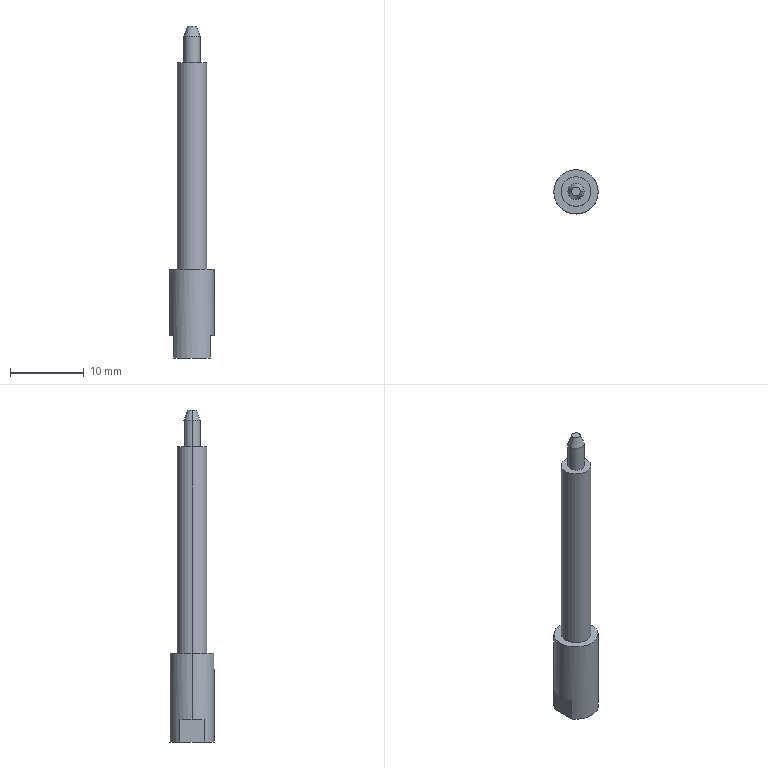Part | STEP file | B09 | 1 solid | 20 faces | box 6 x 6 x 45 mm | volume 663.346 mm3 | cylinder 8 | plane 8 | cone 4 | commonest cylinder face diameters 2.2 x2 2.5 x2 4 x2 6 x2
STEP:
#1=CARTESIAN_POINT('',(0.,0.,0.));
#2=DIRECTION('',(0.,0.,1.));
#3=DIRECTION('',(1.,0.,0.));
#4=AXIS2_PLACEMENT_3D('',#1,#2,#3);
#5=CARTESIAN_POINT('',(-1.25,0.,-4.5));
#6=VERTEX_POINT('',#5);
#7=CARTESIAN_POINT('',(-1.25,0.,-12.));
#8=VERTEX_POINT('',#7);
#9=CARTESIAN_POINT('',(-1.25,0.,-12.));
#10=DIRECTION('',(0.,0.,-1.));
#11=VECTOR('',#10,1.);
#12=LINE('',#9,#11);
#13=CARTESIAN_POINT('',(0.,0.,-12.));
#14=DIRECTION('',(0.,0.,-1.));
#15=DIRECTION('',(-1.,0.,0.));
#16=AXIS2_PLACEMENT_3D('',#13,#14,#15);
#17=CYLINDRICAL_SURFACE('',#16,1.25);
#18=CARTESIAN_POINT('',(6.283,0.));
#19=DIRECTION('',(0.,1.));
#20=VECTOR('',#19,1.);
#21=LINE('',#18,#20);
#22=(GEOMETRIC_REPRESENTATION_CONTEXT(2)PARAMETRIC_REPRESENTATION_CONTEXT()REPRESENTATION_CONTEXT('',''));
#23=DEFINITIONAL_REPRESENTATION('',(#21),#22);
#24=PCURVE('',#17,#23);
#25=CARTESIAN_POINT('',(0.,0.,-12.));
#26=DIRECTION('',(0.,0.,-1.));
#27=DIRECTION('',(-1.,0.,0.));
#28=AXIS2_PLACEMENT_3D('',#25,#26,#27);
#29=CYLINDRICAL_SURFACE('',#28,1.25);
#30=CARTESIAN_POINT('',(0.,0.));
#31=DIRECTION('',(0.,1.));
#32=VECTOR('',#31,1.);
#33=LINE('',#30,#32);
#34=(GEOMETRIC_REPRESENTATION_CONTEXT(2)PARAMETRIC_REPRESENTATION_CONTEXT()REPRESENTATION_CONTEXT('',''));
#35=DEFINITIONAL_REPRESENTATION('',(#33),#34);
#36=PCURVE('',#29,#35);
#37=SURFACE_CURVE('',#12,(#24,#36),.PCURVE_S1.);
#38=EDGE_CURVE('',#6,#8,#37,.T.);
#39=ORIENTED_EDGE('',*,*,#38,.T.);
#40=CARTESIAN_POINT('',(1.25,0.,-12.));
#41=VERTEX_POINT('',#40);
#42=CARTESIAN_POINT('',(0.,0.,-12.));
#43=DIRECTION('',(0.,0.,-1.));
#44=DIRECTION('',(-1.,0.,0.));
#45=AXIS2_PLACEMENT_3D('',#42,#43,#44);
#46=CIRCLE('',#45,1.25);
#47=CARTESIAN_POINT('',(0.,0.));
#48=DIRECTION('',(1.,0.));
#49=VECTOR('',#48,1.);
#50=LINE('',#47,#49);
#51=(GEOMETRIC_REPRESENTATION_CONTEXT(2)PARAMETRIC_REPRESENTATION_CONTEXT()REPRESENTATION_CONTEXT('',''));
#52=DEFINITIONAL_REPRESENTATION('',(#50),#51);
#53=PCURVE('',#17,#52);
#54=CARTESIAN_POINT('',(0.,0.,-12.));
#55=DIRECTION('',(0.,0.,-1.));
#56=DIRECTION('',(-1.,0.,0.));
#57=AXIS2_PLACEMENT_3D('',#54,#55,#56);
#58=PLANE('',#57);
#59=CARTESIAN_POINT('',(0.,0.));
#60=DIRECTION('',(1.,0.));
#61=AXIS2_PLACEMENT_2D('',#59,#60);
#62=CIRCLE('',#61,1.25);
#63=(GEOMETRIC_REPRESENTATION_CONTEXT(2)PARAMETRIC_REPRESENTATION_CONTEXT()REPRESENTATION_CONTEXT('',''));
#64=DEFINITIONAL_REPRESENTATION('',(#62),#63);
#65=PCURVE('',#58,#64);
#66=SURFACE_CURVE('',#46,(#53,#65),.PCURVE_S1.);
#67=EDGE_CURVE('',#41,#8,#66,.T.);
#68=ORIENTED_EDGE('',*,*,#67,.F.);
#69=CARTESIAN_POINT('',(1.25,0.,-4.5));
#70=VERTEX_POINT('',#69);
#71=CARTESIAN_POINT('',(1.25,0.,-12.));
#72=DIRECTION('',(0.,0.,-1.));
#73=VECTOR('',#72,1.);
#74=LINE('',#71,#73);
#75=CARTESIAN_POINT('',(3.142,0.));
#76=DIRECTION('',(0.,1.));
#77=VECTOR('',#76,1.);
#78=LINE('',#75,#77);
#79=(GEOMETRIC_REPRESENTATION_CONTEXT(2)PARAMETRIC_REPRESENTATION_CONTEXT()REPRESENTATION_CONTEXT('',''));
#80=DEFINITIONAL_REPRESENTATION('',(#78),#79);
#81=PCURVE('',#17,#80);
#82=CARTESIAN_POINT('',(3.142,0.));
#83=DIRECTION('',(0.,1.));
#84=VECTOR('',#83,1.);
#85=LINE('',#82,#84);
#86=(GEOMETRIC_REPRESENTATION_CONTEXT(2)PARAMETRIC_REPRESENTATION_CONTEXT()REPRESENTATION_CONTEXT('',''));
#87=DEFINITIONAL_REPRESENTATION('',(#85),#86);
#88=PCURVE('',#29,#87);
#89=SURFACE_CURVE('',#74,(#81,#88),.PCURVE_S1.);
#90=EDGE_CURVE('',#70,#41,#89,.T.);
#91=ORIENTED_EDGE('',*,*,#90,.F.);
#92=CARTESIAN_POINT('',(0.,0.,-4.5));
#93=DIRECTION('',(0.,0.,-1.));
#94=DIRECTION('',(-1.,0.,0.));
#95=AXIS2_PLACEMENT_3D('',#92,#93,#94);
#96=CIRCLE('',#95,1.25);
#97=CARTESIAN_POINT('',(0.,-7.5));
#98=DIRECTION('',(1.,0.));
#99=VECTOR('',#98,1.);
#100=LINE('',#97,#99);
#101=(GEOMETRIC_REPRESENTATION_CONTEXT(2)PARAMETRIC_REPRESENTATION_CONTEXT()REPRESENTATION_CONTEXT('',''));
#102=DEFINITIONAL_REPRESENTATION('',(#100),#101);
#103=PCURVE('',#17,#102);
#104=CARTESIAN_POINT('',(0.,0.,-4.5));
#105=DIRECTION('',(0.,0.,-1.));
#106=DIRECTION('',(-1.,0.,0.));
#107=AXIS2_PLACEMENT_3D('',#104,#105,#106);
#108=CONICAL_SURFACE('',#107,1.25,1.03);
#109=CARTESIAN_POINT('',(0.,0.));
#110=DIRECTION('',(1.,0.));
#111=VECTOR('',#110,1.);
#112=LINE('',#109,#111);
#113=(GEOMETRIC_REPRESENTATION_CONTEXT(2)PARAMETRIC_REPRESENTATION_CONTEXT()REPRESENTATION_CONTEXT('',''));
#114=DEFINITIONAL_REPRESENTATION('',(#112),#113);
#115=PCURVE('',#108,#114);
#116=SURFACE_CURVE('',#96,(#103,#115),.PCURVE_S1.);
#117=EDGE_CURVE('',#70,#6,#116,.T.);
#118=ORIENTED_EDGE('',*,*,#117,.T.);
#119=EDGE_LOOP('',(#39,#68,#91,#118));
#120=FACE_BOUND('',#119,.F.);
#121=ADVANCED_FACE('',(#120),#17,.F.);
#122=ORIENTED_EDGE('',*,*,#117,.F.);
#123=CARTESIAN_POINT('',(0.,0.,-3.749));
#124=VERTEX_POINT('',#123);
#125=CARTESIAN_POINT('',(1.25,0.,-4.5));
#126=DIRECTION('',(0.8572,0.,-0.515));
#127=VECTOR('',#126,1.);
#128=LINE('',#125,#127);
#129=CARTESIAN_POINT('',(3.142,0.));
#130=DIRECTION('',(0.,1.));
#131=VECTOR('',#130,1.);
#132=LINE('',#129,#131);
#133=(GEOMETRIC_REPRESENTATION_CONTEXT(2)PARAMETRIC_REPRESENTATION_CONTEXT()REPRESENTATION_CONTEXT('',''));
#134=DEFINITIONAL_REPRESENTATION('',(#132),#133);
#135=PCURVE('',#108,#134);
#136=CARTESIAN_POINT('',(0.,0.,-4.5));
#137=DIRECTION('',(0.,0.,-1.));
#138=DIRECTION('',(-1.,0.,0.));
#139=AXIS2_PLACEMENT_3D('',#136,#137,#138);
#140=CONICAL_SURFACE('',#139,1.25,1.03);
#141=CARTESIAN_POINT('',(3.142,0.));
#142=DIRECTION('',(0.,1.));
#143=VECTOR('',#142,1.);
#144=LINE('',#141,#143);
#145=(GEOMETRIC_REPRESENTATION_CONTEXT(2)PARAMETRIC_REPRESENTATION_CONTEXT()REPRESENTATION_CONTEXT('',''));
#146=DEFINITIONAL_REPRESENTATION('',(#144),#145);
#147=PCURVE('',#140,#146);
#148=SURFACE_CURVE('',#128,(#135,#147),.PCURVE_S1.);
#149=EDGE_CURVE('',#124,#70,#148,.T.);
#150=ORIENTED_EDGE('',*,*,#149,.F.);
#151=CARTESIAN_POINT('',(-1.25,0.,-4.5));
#152=DIRECTION('',(-0.8572,0.,-0.515));
#153=VECTOR('',#152,1.);
#154=LINE('',#151,#153);
#155=CARTESIAN_POINT('',(6.283,0.));
#156=DIRECTION('',(0.,1.));
#157=VECTOR('',#156,1.);
#158=LINE('',#155,#157);
#159=(GEOMETRIC_REPRESENTATION_CONTEXT(2)PARAMETRIC_REPRESENTATION_CONTEXT()REPRESENTATION_CONTEXT('',''));
#160=DEFINITIONAL_REPRESENTATION('',(#158),#159);
#161=PCURVE('',#108,#160);
#162=CARTESIAN_POINT('',(0.,0.));
#163=DIRECTION('',(0.,1.));
#164=VECTOR('',#163,1.);
#165=LINE('',#162,#164);
#166=(GEOMETRIC_REPRESENTATION_CONTEXT(2)PARAMETRIC_REPRESENTATION_CONTEXT()REPRESENTATION_CONTEXT('',''));
#167=DEFINITIONAL_REPRESENTATION('',(#165),#166);
#168=PCURVE('',#140,#167);
#169=SURFACE_CURVE('',#154,(#161,#168),.PCURVE_S1.);
#170=EDGE_CURVE('',#124,#6,#169,.T.);
#171=ORIENTED_EDGE('',*,*,#170,.T.);
#172=EDGE_LOOP('',(#122,#150,#171));
#173=FACE_BOUND('',#172,.F.);
#174=ADVANCED_FACE('',(#173),#108,.F.);
#175=CARTESIAN_POINT('',(-3.,0.,-9.));
#176=VERTEX_POINT('',#175);
#177=CARTESIAN_POINT('',(-2.5,1.658,-9.));
#178=VERTEX_POINT('',#177);
#179=CARTESIAN_POINT('',(0.,0.,-9.));
#180=DIRECTION('',(0.,0.,-1.));
#181=DIRECTION('',(-1.,0.,0.));
#182=AXIS2_PLACEMENT_3D('',#179,#180,#181);
#183=CIRCLE('',#182,3.);
#184=CARTESIAN_POINT('',(0.,0.,-12.));
#185=DIRECTION('',(0.,0.,1.));
#186=DIRECTION('',(1.,0.,0.));
#187=AXIS2_PLACEMENT_3D('',#184,#185,#186);
#188=CYLINDRICAL_SURFACE('',#187,3.);
#189=CARTESIAN_POINT('',(3.142,3.));
#190=DIRECTION('',(-1.,0.));
#191=VECTOR('',#190,1.);
#192=LINE('',#189,#191);
#193=(GEOMETRIC_REPRESENTATION_CONTEXT(2)PARAMETRIC_REPRESENTATION_CONTEXT()REPRESENTATION_CONTEXT('',''));
#194=DEFINITIONAL_REPRESENTATION('',(#192),#193);
#195=PCURVE('',#188,#194);
#196=CARTESIAN_POINT('',(0.,0.,-9.));
#197=DIRECTION('',(0.,0.,-1.));
#198=DIRECTION('',(-1.,0.,0.));
#199=AXIS2_PLACEMENT_3D('',#196,#197,#198);
#200=PLANE('',#199);
#201=CARTESIAN_POINT('',(0.,0.));
#202=DIRECTION('',(1.,0.));
#203=AXIS2_PLACEMENT_2D('',#201,#202);
#204=CIRCLE('',#203,3.);
#205=(GEOMETRIC_REPRESENTATION_CONTEXT(2)PARAMETRIC_REPRESENTATION_CONTEXT()REPRESENTATION_CONTEXT('',''));
#206=DEFINITIONAL_REPRESENTATION('',(#204),#205);
#207=PCURVE('',#200,#206);
#208=SURFACE_CURVE('',#183,(#195,#207),.PCURVE_S1.);
#209=EDGE_CURVE('',#176,#178,#208,.T.);
#210=ORIENTED_EDGE('',*,*,#209,.F.);
#211=CARTESIAN_POINT('',(-3.,0.,0.));
#212=VERTEX_POINT('',#211);
#213=CARTESIAN_POINT('',(-3.,0.,-12.));
#214=DIRECTION('',(0.,0.,1.));
#215=VECTOR('',#214,1.);
#216=LINE('',#213,#215);
#217=CARTESIAN_POINT('',(3.142,0.));
#218=DIRECTION('',(0.,1.));
#219=VECTOR('',#218,1.);
#220=LINE('',#217,#219);
#221=(GEOMETRIC_REPRESENTATION_CONTEXT(2)PARAMETRIC_REPRESENTATION_CONTEXT()REPRESENTATION_CONTEXT('',''));
#222=DEFINITIONAL_REPRESENTATION('',(#220),#221);
#223=PCURVE('',#188,#222);
#224=CARTESIAN_POINT('',(0.,0.,-12.));
#225=DIRECTION('',(0.,0.,1.));
#226=DIRECTION('',(1.,0.,0.));
#227=AXIS2_PLACEMENT_3D('',#224,#225,#226);
#228=CYLINDRICAL_SURFACE('',#227,3.);
#229=CARTESIAN_POINT('',(3.142,0.));
#230=DIRECTION('',(0.,1.));
#231=VECTOR('',#230,1.);
#232=LINE('',#229,#231);
#233=(GEOMETRIC_REPRESENTATION_CONTEXT(2)PARAMETRIC_REPRESENTATION_CONTEXT()REPRESENTATION_CONTEXT('',''));
#234=DEFINITIONAL_REPRESENTATION('',(#232),#233);
#235=PCURVE('',#228,#234);
#236=SURFACE_CURVE('',#216,(#223,#235),.PCURVE_S1.);
#237=EDGE_CURVE('',#176,#212,#236,.T.);
#238=ORIENTED_EDGE('',*,*,#237,.T.);
#239=CARTESIAN_POINT('',(3.,0.,0.));
#240=VERTEX_POINT('',#239);
#241=CARTESIAN_POINT('',(0.,0.,0.));
#242=DIRECTION('',(0.,0.,-1.));
#243=DIRECTION('',(-1.,0.,0.));
#244=AXIS2_PLACEMENT_3D('',#241,#242,#243);
#245=CIRCLE('',#244,3.);
#246=CARTESIAN_POINT('',(3.142,12.));
#247=DIRECTION('',(-1.,0.));
#248=VECTOR('',#247,1.);
#249=LINE('',#246,#248);
#250=(GEOMETRIC_REPRESENTATION_CONTEXT(2)PARAMETRIC_REPRESENTATION_CONTEXT()REPRESENTATION_CONTEXT('',''));
#251=DEFINITIONAL_REPRESENTATION('',(#249),#250);
#252=PCURVE('',#188,#251);
#253=CARTESIAN_POINT('',(0.,0.,0.));
#254=DIRECTION('',(0.,0.,-1.));
#255=DIRECTION('',(-1.,0.,0.));
#256=AXIS2_PLACEMENT_3D('',#253,#254,#255);
#257=PLANE('',#256);
#258=CARTESIAN_POINT('',(0.,0.));
#259=DIRECTION('',(1.,0.));
#260=AXIS2_PLACEMENT_2D('',#258,#259);
#261=CIRCLE('',#260,3.);
#262=(GEOMETRIC_REPRESENTATION_CONTEXT(2)PARAMETRIC_REPRESENTATION_CONTEXT()REPRESENTATION_CONTEXT('',''));
#263=DEFINITIONAL_REPRESENTATION('',(#261),#262);
#264=PCURVE('',#257,#263);
#265=SURFACE_CURVE('',#245,(#252,#264),.PCURVE_S1.);
#266=EDGE_CURVE('',#212,#240,#265,.T.);
#267=ORIENTED_EDGE('',*,*,#266,.T.);
#268=CARTESIAN_POINT('',(3.,0.,-9.));
#269=VERTEX_POINT('',#268);
#270=CARTESIAN_POINT('',(3.,0.,-12.));
#271=DIRECTION('',(0.,0.,1.));
#272=VECTOR('',#271,1.);
#273=LINE('',#270,#272);
#274=CARTESIAN_POINT('',(0.,0.));
#275=DIRECTION('',(0.,1.));
#276=VECTOR('',#275,1.);
#277=LINE('',#274,#276);
#278=(GEOMETRIC_REPRESENTATION_CONTEXT(2)PARAMETRIC_REPRESENTATION_CONTEXT()REPRESENTATION_CONTEXT('',''));
#279=DEFINITIONAL_REPRESENTATION('',(#277),#278);
#280=PCURVE('',#188,#279);
#281=CARTESIAN_POINT('',(6.283,0.));
#282=DIRECTION('',(0.,1.));
#283=VECTOR('',#282,1.);
#284=LINE('',#281,#283);
#285=(GEOMETRIC_REPRESENTATION_CONTEXT(2)PARAMETRIC_REPRESENTATION_CONTEXT()REPRESENTATION_CONTEXT('',''));
#286=DEFINITIONAL_REPRESENTATION('',(#284),#285);
#287=PCURVE('',#228,#286);
#288=SURFACE_CURVE('',#273,(#280,#287),.PCURVE_S1.);
#289=EDGE_CURVE('',#269,#240,#288,.T.);
#290=ORIENTED_EDGE('',*,*,#289,.F.);
#291=CARTESIAN_POINT('',(2.5,1.658,-9.));
#292=VERTEX_POINT('',#291);
#293=CARTESIAN_POINT('',(0.,0.,-9.));
#294=DIRECTION('',(0.,0.,-1.));
#295=DIRECTION('',(-1.,0.,0.));
#296=AXIS2_PLACEMENT_3D('',#293,#294,#295);
#297=CIRCLE('',#296,3.);
#298=CARTESIAN_POINT('',(3.142,3.));
#299=DIRECTION('',(-1.,0.));
#300=VECTOR('',#299,1.);
#301=LINE('',#298,#300);
#302=(GEOMETRIC_REPRESENTATION_CONTEXT(2)PARAMETRIC_REPRESENTATION_CONTEXT()REPRESENTATION_CONTEXT('',''));
#303=DEFINITIONAL_REPRESENTATION('',(#301),#302);
#304=PCURVE('',#188,#303);
#305=CARTESIAN_POINT('',(0.,0.,-9.));
#306=DIRECTION('',(0.,0.,-1.));
#307=DIRECTION('',(-1.,0.,0.));
#308=AXIS2_PLACEMENT_3D('',#305,#306,#307);
#309=PLANE('',#308);
#310=CARTESIAN_POINT('',(0.,0.));
#311=DIRECTION('',(1.,0.));
#312=AXIS2_PLACEMENT_2D('',#310,#311);
#313=CIRCLE('',#312,3.);
#314=(GEOMETRIC_REPRESENTATION_CONTEXT(2)PARAMETRIC_REPRESENTATION_CONTEXT()REPRESENTATION_CONTEXT('',''));
#315=DEFINITIONAL_REPRESENTATION('',(#313),#314);
#316=PCURVE('',#309,#315);
#317=SURFACE_CURVE('',#297,(#304,#316),.PCURVE_S1.);
#318=EDGE_CURVE('',#292,#269,#317,.T.);
#319=ORIENTED_EDGE('',*,*,#318,.F.);
#320=CARTESIAN_POINT('',(2.5,1.658,-12.));
#321=VERTEX_POINT('',#320);
#322=CARTESIAN_POINT('',(2.5,1.658,-12.));
#323=DIRECTION('',(0.,0.,-1.));
#324=VECTOR('',#323,1.);
#325=LINE('',#322,#324);
#326=CARTESIAN_POINT('',(0.5857,0.));
#327=DIRECTION('',(0.,-1.));
#328=VECTOR('',#327,1.);
#329=LINE('',#326,#328);
#330=(GEOMETRIC_REPRESENTATION_CONTEXT(2)PARAMETRIC_REPRESENTATION_CONTEXT()REPRESENTATION_CONTEXT('',''));
#331=DEFINITIONAL_REPRESENTATION('',(#329),#330);
#332=PCURVE('',#188,#331);
#333=CARTESIAN_POINT('',(2.5,3.681,-9.));
#334=DIRECTION('',(-1.,0.,0.));
#335=DIRECTION('',(0.,-1.,0.));
#336=AXIS2_PLACEMENT_3D('',#333,#334,#335);
#337=PLANE('',#336);
#338=CARTESIAN_POINT('',(2.023,-3.));
#339=DIRECTION('',(0.,-1.));
#340=VECTOR('',#339,1.);
#341=LINE('',#338,#340);
#342=(GEOMETRIC_REPRESENTATION_CONTEXT(2)PARAMETRIC_REPRESENTATION_CONTEXT()REPRESENTATION_CONTEXT('',''));
#343=DEFINITIONAL_REPRESENTATION('',(#341),#342);
#344=PCURVE('',#337,#343);
#345=SURFACE_CURVE('',#325,(#332,#344),.PCURVE_S1.);
#346=EDGE_CURVE('',#292,#321,#345,.T.);
#347=ORIENTED_EDGE('',*,*,#346,.T.);
#348=CARTESIAN_POINT('',(-2.5,1.658,-12.));
#349=VERTEX_POINT('',#348);
#350=CARTESIAN_POINT('',(0.,0.,-12.));
#351=DIRECTION('',(0.,0.,-1.));
#352=DIRECTION('',(-1.,0.,0.));
#353=AXIS2_PLACEMENT_3D('',#350,#351,#352);
#354=CIRCLE('',#353,3.);
#355=CARTESIAN_POINT('',(3.142,0.));
#356=DIRECTION('',(-1.,0.));
#357=VECTOR('',#356,1.);
#358=LINE('',#355,#357);
#359=(GEOMETRIC_REPRESENTATION_CONTEXT(2)PARAMETRIC_REPRESENTATION_CONTEXT()REPRESENTATION_CONTEXT('',''));
#360=DEFINITIONAL_REPRESENTATION('',(#358),#359);
#361=PCURVE('',#188,#360);
#362=CARTESIAN_POINT('',(0.,0.));
#363=DIRECTION('',(1.,0.));
#364=AXIS2_PLACEMENT_2D('',#362,#363);
#365=CIRCLE('',#364,3.);
#366=(GEOMETRIC_REPRESENTATION_CONTEXT(2)PARAMETRIC_REPRESENTATION_CONTEXT()REPRESENTATION_CONTEXT('',''));
#367=DEFINITIONAL_REPRESENTATION('',(#365),#366);
#368=PCURVE('',#58,#367);
#369=SURFACE_CURVE('',#354,(#361,#368),.PCURVE_S1.);
#370=EDGE_CURVE('',#349,#321,#369,.T.);
#371=ORIENTED_EDGE('',*,*,#370,.F.);
#372=CARTESIAN_POINT('',(-2.5,1.658,-12.));
#373=DIRECTION('',(0.,0.,1.));
#374=VECTOR('',#373,1.);
#375=LINE('',#372,#374);
#376=CARTESIAN_POINT('',(2.556,0.));
#377=DIRECTION('',(0.,1.));
#378=VECTOR('',#377,1.);
#379=LINE('',#376,#378);
#380=(GEOMETRIC_REPRESENTATION_CONTEXT(2)PARAMETRIC_REPRESENTATION_CONTEXT()REPRESENTATION_CONTEXT('',''));
#381=DEFINITIONAL_REPRESENTATION('',(#379),#380);
#382=PCURVE('',#188,#381);
#383=CARTESIAN_POINT('',(-2.5,-4.861,-9.));
#384=DIRECTION('',(1.,0.,0.));
#385=DIRECTION('',(0.,0.,-1.));
#386=AXIS2_PLACEMENT_3D('',#383,#384,#385);
#387=PLANE('',#386);
#388=CARTESIAN_POINT('',(3.,6.52));
#389=DIRECTION('',(-1.,0.));
#390=VECTOR('',#389,1.);
#391=LINE('',#388,#390);
#392=(GEOMETRIC_REPRESENTATION_CONTEXT(2)PARAMETRIC_REPRESENTATION_CONTEXT()REPRESENTATION_CONTEXT('',''));
#393=DEFINITIONAL_REPRESENTATION('',(#391),#392);
#394=PCURVE('',#387,#393);
#395=SURFACE_CURVE('',#375,(#382,#394),.PCURVE_S1.);
#396=EDGE_CURVE('',#349,#178,#395,.T.);
#397=ORIENTED_EDGE('',*,*,#396,.T.);
#398=EDGE_LOOP('',(#210,#238,#267,#290,#319,#347,#371,#397));
#399=FACE_BOUND('',#398,.T.);
#400=ADVANCED_FACE('',(#399),#188,.T.);
#401=CARTESIAN_POINT('',(0.6,0.,33.));
#402=VERTEX_POINT('',#401);
#403=CARTESIAN_POINT('',(-0.6,0.,33.));
#404=VERTEX_POINT('',#403);
#405=CARTESIAN_POINT('',(0.,0.,33.));
#406=DIRECTION('',(0.,0.,1.));
#407=DIRECTION('',(1.,0.,0.));
#408=AXIS2_PLACEMENT_3D('',#405,#406,#407);
#409=CIRCLE('',#408,0.6);
#410=CARTESIAN_POINT('',(0.,0.,33.));
#411=DIRECTION('',(0.,0.,-1.));
#412=DIRECTION('',(-1.,0.,0.));
#413=AXIS2_PLACEMENT_3D('',#410,#411,#412);
#414=CONICAL_SURFACE('',#413,0.6,0.3491);
#415=CARTESIAN_POINT('',(3.142,0.));
#416=DIRECTION('',(-1.,0.));
#417=VECTOR('',#416,1.);
#418=LINE('',#415,#417);
#419=(GEOMETRIC_REPRESENTATION_CONTEXT(2)PARAMETRIC_REPRESENTATION_CONTEXT()REPRESENTATION_CONTEXT('',''));
#420=DEFINITIONAL_REPRESENTATION('',(#418),#419);
#421=PCURVE('',#414,#420);
#422=CARTESIAN_POINT('',(0.,0.,33.));
#423=DIRECTION('',(0.,0.,1.));
#424=DIRECTION('',(1.,0.,0.));
#425=AXIS2_PLACEMENT_3D('',#422,#423,#424);
#426=PLANE('',#425);
#427=CARTESIAN_POINT('',(0.,0.));
#428=DIRECTION('',(1.,0.));
#429=AXIS2_PLACEMENT_2D('',#427,#428);
#430=CIRCLE('',#429,0.6);
#431=(GEOMETRIC_REPRESENTATION_CONTEXT(2)PARAMETRIC_REPRESENTATION_CONTEXT()REPRESENTATION_CONTEXT('',''));
#432=DEFINITIONAL_REPRESENTATION('',(#430),#431);
#433=PCURVE('',#426,#432);
#434=SURFACE_CURVE('',#409,(#421,#433),.PCURVE_S1.);
#435=EDGE_CURVE('',#402,#404,#434,.T.);
#436=ORIENTED_EDGE('',*,*,#435,.F.);
#437=CARTESIAN_POINT('',(1.1,0.,31.626));
#438=VERTEX_POINT('',#437);
#439=CARTESIAN_POINT('',(0.6,0.,33.));
#440=DIRECTION('',(0.342,0.,-0.9397));
#441=VECTOR('',#440,1.);
#442=LINE('',#439,#441);
#443=CARTESIAN_POINT('',(3.142,0.));
#444=DIRECTION('',(0.,1.));
#445=VECTOR('',#444,1.);
#446=LINE('',#443,#445);
#447=(GEOMETRIC_REPRESENTATION_CONTEXT(2)PARAMETRIC_REPRESENTATION_CONTEXT()REPRESENTATION_CONTEXT('',''));
#448=DEFINITIONAL_REPRESENTATION('',(#446),#447);
#449=PCURVE('',#414,#448);
#450=CARTESIAN_POINT('',(0.,0.,33.));
#451=DIRECTION('',(0.,0.,-1.));
#452=DIRECTION('',(-1.,0.,0.));
#453=AXIS2_PLACEMENT_3D('',#450,#451,#452);
#454=CONICAL_SURFACE('',#453,0.6,0.3491);
#455=CARTESIAN_POINT('',(3.142,0.));
#456=DIRECTION('',(0.,1.));
#457=VECTOR('',#456,1.);
#458=LINE('',#455,#457);
#459=(GEOMETRIC_REPRESENTATION_CONTEXT(2)PARAMETRIC_REPRESENTATION_CONTEXT()REPRESENTATION_CONTEXT('',''));
#460=DEFINITIONAL_REPRESENTATION('',(#458),#459);
#461=PCURVE('',#454,#460);
#462=SURFACE_CURVE('',#442,(#449,#461),.PCURVE_S1.);
#463=EDGE_CURVE('',#402,#438,#462,.T.);
#464=ORIENTED_EDGE('',*,*,#463,.T.);
#465=CARTESIAN_POINT('',(-1.1,0.,31.626));
#466=VERTEX_POINT('',#465);
#467=CARTESIAN_POINT('',(0.,0.,31.626));
#468=DIRECTION('',(0.,0.,-1.));
#469=DIRECTION('',(1.,0.,0.));
#470=AXIS2_PLACEMENT_3D('',#467,#468,#469);
#471=CIRCLE('',#470,1.1);
#472=CARTESIAN_POINT('',(-3.142,1.374));
#473=DIRECTION('',(1.,0.));
#474=VECTOR('',#473,1.);
#475=LINE('',#472,#474);
#476=(GEOMETRIC_REPRESENTATION_CONTEXT(2)PARAMETRIC_REPRESENTATION_CONTEXT()REPRESENTATION_CONTEXT('',''));
#477=DEFINITIONAL_REPRESENTATION('',(#475),#476);
#478=PCURVE('',#414,#477);
#479=CARTESIAN_POINT('',(0.,0.,33.));
#480=DIRECTION('',(0.,0.,-1.));
#481=DIRECTION('',(-1.,0.,0.));
#482=AXIS2_PLACEMENT_3D('',#479,#480,#481);
#483=CYLINDRICAL_SURFACE('',#482,1.1);
#484=CARTESIAN_POINT('',(-3.142,1.374));
#485=DIRECTION('',(1.,0.));
#486=VECTOR('',#485,1.);
#487=LINE('',#484,#486);
#488=(GEOMETRIC_REPRESENTATION_CONTEXT(2)PARAMETRIC_REPRESENTATION_CONTEXT()REPRESENTATION_CONTEXT('',''));
#489=DEFINITIONAL_REPRESENTATION('',(#487),#488);
#490=PCURVE('',#483,#489);
#491=SURFACE_CURVE('',#471,(#478,#490),.PCURVE_S1.);
#492=EDGE_CURVE('',#466,#438,#491,.T.);
#493=ORIENTED_EDGE('',*,*,#492,.F.);
#494=CARTESIAN_POINT('',(-0.6,0.,33.));
#495=DIRECTION('',(-0.342,0.,-0.9397));
#496=VECTOR('',#495,1.);
#497=LINE('',#494,#496);
#498=CARTESIAN_POINT('',(0.,0.));
#499=DIRECTION('',(0.,1.));
#500=VECTOR('',#499,1.);
#501=LINE('',#498,#500);
#502=(GEOMETRIC_REPRESENTATION_CONTEXT(2)PARAMETRIC_REPRESENTATION_CONTEXT()REPRESENTATION_CONTEXT('',''));
#503=DEFINITIONAL_REPRESENTATION('',(#501),#502);
#504=PCURVE('',#414,#503);
#505=CARTESIAN_POINT('',(6.283,0.));
#506=DIRECTION('',(0.,1.));
#507=VECTOR('',#506,1.);
#508=LINE('',#505,#507);
#509=(GEOMETRIC_REPRESENTATION_CONTEXT(2)PARAMETRIC_REPRESENTATION_CONTEXT()REPRESENTATION_CONTEXT('',''));
#510=DEFINITIONAL_REPRESENTATION('',(#508),#509);
#511=PCURVE('',#454,#510);
#512=SURFACE_CURVE('',#497,(#504,#511),.PCURVE_S1.);
#513=EDGE_CURVE('',#404,#466,#512,.T.);
#514=ORIENTED_EDGE('',*,*,#513,.F.);
#515=EDGE_LOOP('',(#436,#464,#493,#514));
#516=FACE_BOUND('',#515,.T.);
#517=ADVANCED_FACE('',(#516),#414,.T.);
#518=ORIENTED_EDGE('',*,*,#492,.T.);
#519=CARTESIAN_POINT('',(1.1,0.,28.));
#520=VERTEX_POINT('',#519);
#521=CARTESIAN_POINT('',(1.1,0.,33.));
#522=DIRECTION('',(0.,0.,-1.));
#523=VECTOR('',#522,1.);
#524=LINE('',#521,#523);
#525=CARTESIAN_POINT('',(3.142,0.));
#526=DIRECTION('',(0.,1.));
#527=VECTOR('',#526,1.);
#528=LINE('',#525,#527);
#529=(GEOMETRIC_REPRESENTATION_CONTEXT(2)PARAMETRIC_REPRESENTATION_CONTEXT()REPRESENTATION_CONTEXT('',''));
#530=DEFINITIONAL_REPRESENTATION('',(#528),#529);
#531=PCURVE('',#483,#530);
#532=CARTESIAN_POINT('',(0.,0.,33.));
#533=DIRECTION('',(0.,0.,-1.));
#534=DIRECTION('',(-1.,0.,0.));
#535=AXIS2_PLACEMENT_3D('',#532,#533,#534);
#536=CYLINDRICAL_SURFACE('',#535,1.1);
#537=CARTESIAN_POINT('',(3.142,0.));
#538=DIRECTION('',(0.,1.));
#539=VECTOR('',#538,1.);
#540=LINE('',#537,#539);
#541=(GEOMETRIC_REPRESENTATION_CONTEXT(2)PARAMETRIC_REPRESENTATION_CONTEXT()REPRESENTATION_CONTEXT('',''));
#542=DEFINITIONAL_REPRESENTATION('',(#540),#541);
#543=PCURVE('',#536,#542);
#544=SURFACE_CURVE('',#524,(#531,#543),.PCURVE_S1.);
#545=EDGE_CURVE('',#438,#520,#544,.T.);
#546=ORIENTED_EDGE('',*,*,#545,.T.);
#547=CARTESIAN_POINT('',(-1.1,0.,28.));
#548=VERTEX_POINT('',#547);
#549=CARTESIAN_POINT('',(0.,0.,28.));
#550=DIRECTION('',(0.,0.,1.));
#551=DIRECTION('',(1.,0.,0.));
#552=AXIS2_PLACEMENT_3D('',#549,#550,#551);
#553=CIRCLE('',#552,1.1);
#554=CARTESIAN_POINT('',(3.142,5.));
#555=DIRECTION('',(-1.,0.));
#556=VECTOR('',#555,1.);
#557=LINE('',#554,#556);
#558=(GEOMETRIC_REPRESENTATION_CONTEXT(2)PARAMETRIC_REPRESENTATION_CONTEXT()REPRESENTATION_CONTEXT('',''));
#559=DEFINITIONAL_REPRESENTATION('',(#557),#558);
#560=PCURVE('',#483,#559);
#561=CARTESIAN_POINT('',(0.,0.,28.));
#562=DIRECTION('',(0.,0.,1.));
#563=DIRECTION('',(1.,0.,0.));
#564=AXIS2_PLACEMENT_3D('',#561,#562,#563);
#565=PLANE('',#564);
#566=CARTESIAN_POINT('',(0.,0.));
#567=DIRECTION('',(1.,0.));
#568=AXIS2_PLACEMENT_2D('',#566,#567);
#569=CIRCLE('',#568,1.1);
#570=(GEOMETRIC_REPRESENTATION_CONTEXT(2)PARAMETRIC_REPRESENTATION_CONTEXT()REPRESENTATION_CONTEXT('',''));
#571=DEFINITIONAL_REPRESENTATION('',(#569),#570);
#572=PCURVE('',#565,#571);
#573=SURFACE_CURVE('',#553,(#560,#572),.PCURVE_S1.);
#574=EDGE_CURVE('',#520,#548,#573,.T.);
#575=ORIENTED_EDGE('',*,*,#574,.T.);
#576=CARTESIAN_POINT('',(-1.1,0.,33.));
#577=DIRECTION('',(0.,0.,-1.));
#578=VECTOR('',#577,1.);
#579=LINE('',#576,#578);
#580=CARTESIAN_POINT('',(0.,0.));
#581=DIRECTION('',(0.,1.));
#582=VECTOR('',#581,1.);
#583=LINE('',#580,#582);
#584=(GEOMETRIC_REPRESENTATION_CONTEXT(2)PARAMETRIC_REPRESENTATION_CONTEXT()REPRESENTATION_CONTEXT('',''));
#585=DEFINITIONAL_REPRESENTATION('',(#583),#584);
#586=PCURVE('',#483,#585);
#587=CARTESIAN_POINT('',(6.283,0.));
#588=DIRECTION('',(0.,1.));
#589=VECTOR('',#588,1.);
#590=LINE('',#587,#589);
#591=(GEOMETRIC_REPRESENTATION_CONTEXT(2)PARAMETRIC_REPRESENTATION_CONTEXT()REPRESENTATION_CONTEXT('',''));
#592=DEFINITIONAL_REPRESENTATION('',(#590),#591);
#593=PCURVE('',#536,#592);
#594=SURFACE_CURVE('',#579,(#586,#593),.PCURVE_S1.);
#595=EDGE_CURVE('',#466,#548,#594,.T.);
#596=ORIENTED_EDGE('',*,*,#595,.F.);
#597=EDGE_LOOP('',(#518,#546,#575,#596));
#598=FACE_BOUND('',#597,.T.);
#599=ADVANCED_FACE('',(#598),#483,.T.);
#600=CARTESIAN_POINT('',(2.,0.,28.));
#601=VERTEX_POINT('',#600);
#602=CARTESIAN_POINT('',(-2.,0.,28.));
#603=VERTEX_POINT('',#602);
#604=CARTESIAN_POINT('',(0.,0.,28.));
#605=DIRECTION('',(0.,0.,1.));
#606=DIRECTION('',(1.,0.,0.));
#607=AXIS2_PLACEMENT_3D('',#604,#605,#606);
#608=CIRCLE('',#607,2.);
#609=CARTESIAN_POINT('',(0.,0.,28.));
#610=DIRECTION('',(0.,0.,-1.));
#611=DIRECTION('',(-1.,0.,0.));
#612=AXIS2_PLACEMENT_3D('',#609,#610,#611);
#613=CYLINDRICAL_SURFACE('',#612,2.);
#614=CARTESIAN_POINT('',(3.142,0.));
#615=DIRECTION('',(-1.,0.));
#616=VECTOR('',#615,1.);
#617=LINE('',#614,#616);
#618=(GEOMETRIC_REPRESENTATION_CONTEXT(2)PARAMETRIC_REPRESENTATION_CONTEXT()REPRESENTATION_CONTEXT('',''));
#619=DEFINITIONAL_REPRESENTATION('',(#617),#618);
#620=PCURVE('',#613,#619);
#621=CARTESIAN_POINT('',(0.,0.));
#622=DIRECTION('',(1.,0.));
#623=AXIS2_PLACEMENT_2D('',#621,#622);
#624=CIRCLE('',#623,2.);
#625=(GEOMETRIC_REPRESENTATION_CONTEXT(2)PARAMETRIC_REPRESENTATION_CONTEXT()REPRESENTATION_CONTEXT('',''));
#626=DEFINITIONAL_REPRESENTATION('',(#624),#625);
#627=PCURVE('',#565,#626);
#628=SURFACE_CURVE('',#608,(#620,#627),.PCURVE_S1.);
#629=EDGE_CURVE('',#601,#603,#628,.T.);
#630=ORIENTED_EDGE('',*,*,#629,.F.);
#631=CARTESIAN_POINT('',(2.,0.,0.));
#632=VERTEX_POINT('',#631);
#633=CARTESIAN_POINT('',(2.,0.,28.));
#634=DIRECTION('',(0.,0.,-1.));
#635=VECTOR('',#634,1.);
#636=LINE('',#633,#635);
#637=CARTESIAN_POINT('',(3.142,0.));
#638=DIRECTION('',(0.,1.));
#639=VECTOR('',#638,1.);
#640=LINE('',#637,#639);
#641=(GEOMETRIC_REPRESENTATION_CONTEXT(2)PARAMETRIC_REPRESENTATION_CONTEXT()REPRESENTATION_CONTEXT('',''));
#642=DEFINITIONAL_REPRESENTATION('',(#640),#641);
#643=PCURVE('',#613,#642);
#644=CARTESIAN_POINT('',(0.,0.,28.));
#645=DIRECTION('',(0.,0.,-1.));
#646=DIRECTION('',(-1.,0.,0.));
#647=AXIS2_PLACEMENT_3D('',#644,#645,#646);
#648=CYLINDRICAL_SURFACE('',#647,2.);
#649=CARTESIAN_POINT('',(3.142,0.));
#650=DIRECTION('',(0.,1.));
#651=VECTOR('',#650,1.);
#652=LINE('',#649,#651);
#653=(GEOMETRIC_REPRESENTATION_CONTEXT(2)PARAMETRIC_REPRESENTATION_CONTEXT()REPRESENTATION_CONTEXT('',''));
#654=DEFINITIONAL_REPRESENTATION('',(#652),#653);
#655=PCURVE('',#648,#654);
#656=SURFACE_CURVE('',#636,(#643,#655),.PCURVE_S1.);
#657=EDGE_CURVE('',#601,#632,#656,.T.);
#658=ORIENTED_EDGE('',*,*,#657,.T.);
#659=CARTESIAN_POINT('',(-2.,0.,0.));
#660=VERTEX_POINT('',#659);
#661=CARTESIAN_POINT('',(0.,0.,0.));
#662=DIRECTION('',(0.,0.,-1.));
#663=DIRECTION('',(-1.,0.,0.));
#664=AXIS2_PLACEMENT_3D('',#661,#662,#663);
#665=CIRCLE('',#664,2.);
#666=CARTESIAN_POINT('',(0.,28.));
#667=DIRECTION('',(1.,0.));
#668=VECTOR('',#667,1.);
#669=LINE('',#666,#668);
#670=(GEOMETRIC_REPRESENTATION_CONTEXT(2)PARAMETRIC_REPRESENTATION_CONTEXT()REPRESENTATION_CONTEXT('',''));
#671=DEFINITIONAL_REPRESENTATION('',(#669),#670);
#672=PCURVE('',#613,#671);
#673=CARTESIAN_POINT('',(0.,0.));
#674=DIRECTION('',(1.,0.));
#675=AXIS2_PLACEMENT_2D('',#673,#674);
#676=CIRCLE('',#675,2.);
#677=(GEOMETRIC_REPRESENTATION_CONTEXT(2)PARAMETRIC_REPRESENTATION_CONTEXT()REPRESENTATION_CONTEXT('',''));
#678=DEFINITIONAL_REPRESENTATION('',(#676),#677);
#679=PCURVE('',#257,#678);
#680=SURFACE_CURVE('',#665,(#672,#679),.PCURVE_S1.);
#681=EDGE_CURVE('',#660,#632,#680,.T.);
#682=ORIENTED_EDGE('',*,*,#681,.F.);
#683=CARTESIAN_POINT('',(-2.,0.,28.));
#684=DIRECTION('',(0.,0.,-1.));
#685=VECTOR('',#684,1.);
#686=LINE('',#683,#685);
#687=CARTESIAN_POINT('',(0.,0.));
#688=DIRECTION('',(0.,1.));
#689=VECTOR('',#688,1.);
#690=LINE('',#687,#689);
#691=(GEOMETRIC_REPRESENTATION_CONTEXT(2)PARAMETRIC_REPRESENTATION_CONTEXT()REPRESENTATION_CONTEXT('',''));
#692=DEFINITIONAL_REPRESENTATION('',(#690),#691);
#693=PCURVE('',#613,#692);
#694=CARTESIAN_POINT('',(6.283,0.));
#695=DIRECTION('',(0.,1.));
#696=VECTOR('',#695,1.);
#697=LINE('',#694,#696);
#698=(GEOMETRIC_REPRESENTATION_CONTEXT(2)PARAMETRIC_REPRESENTATION_CONTEXT()REPRESENTATION_CONTEXT('',''));
#699=DEFINITIONAL_REPRESENTATION('',(#697),#698);
#700=PCURVE('',#648,#699);
#701=SURFACE_CURVE('',#686,(#693,#700),.PCURVE_S1.);
#702=EDGE_CURVE('',#603,#660,#701,.T.);
#703=ORIENTED_EDGE('',*,*,#702,.F.);
#704=EDGE_LOOP('',(#630,#658,#682,#703));
#705=FACE_BOUND('',#704,.T.);
#706=ADVANCED_FACE('',(#705),#613,.T.);
#707=CARTESIAN_POINT('',(0.,0.,28.));
#708=DIRECTION('',(0.,0.,1.));
#709=DIRECTION('',(1.,0.,0.));
#710=AXIS2_PLACEMENT_3D('',#707,#708,#709);
#711=CIRCLE('',#710,2.);
#712=CARTESIAN_POINT('',(0.,0.));
#713=DIRECTION('',(1.,0.));
#714=AXIS2_PLACEMENT_2D('',#712,#713);
#715=CIRCLE('',#714,2.);
#716=(GEOMETRIC_REPRESENTATION_CONTEXT(2)PARAMETRIC_REPRESENTATION_CONTEXT()REPRESENTATION_CONTEXT('',''));
#717=DEFINITIONAL_REPRESENTATION('',(#715),#716);
#718=PCURVE('',#565,#717);
#719=CARTESIAN_POINT('',(9.425,0.));
#720=DIRECTION('',(-1.,0.));
#721=VECTOR('',#720,1.);
#722=LINE('',#719,#721);
#723=(GEOMETRIC_REPRESENTATION_CONTEXT(2)PARAMETRIC_REPRESENTATION_CONTEXT()REPRESENTATION_CONTEXT('',''));
#724=DEFINITIONAL_REPRESENTATION('',(#722),#723);
#725=PCURVE('',#648,#724);
#726=SURFACE_CURVE('',#711,(#718,#725),.PCURVE_S1.);
#727=EDGE_CURVE('',#603,#601,#726,.T.);
#728=ORIENTED_EDGE('',*,*,#727,.T.);
#729=ORIENTED_EDGE('',*,*,#629,.T.);
#730=EDGE_LOOP('',(#728,#729));
#731=FACE_BOUND('',#730,.T.);
#732=CARTESIAN_POINT('',(0.,0.,28.));
#733=DIRECTION('',(0.,0.,1.));
#734=DIRECTION('',(1.,0.,0.));
#735=AXIS2_PLACEMENT_3D('',#732,#733,#734);
#736=CIRCLE('',#735,1.1);
#737=CARTESIAN_POINT('',(0.,0.));
#738=DIRECTION('',(1.,0.));
#739=AXIS2_PLACEMENT_2D('',#737,#738);
#740=CIRCLE('',#739,1.1);
#741=(GEOMETRIC_REPRESENTATION_CONTEXT(2)PARAMETRIC_REPRESENTATION_CONTEXT()REPRESENTATION_CONTEXT('',''));
#742=DEFINITIONAL_REPRESENTATION('',(#740),#741);
#743=PCURVE('',#565,#742);
#744=CARTESIAN_POINT('',(9.425,5.));
#745=DIRECTION('',(-1.,0.));
#746=VECTOR('',#745,1.);
#747=LINE('',#744,#746);
#748=(GEOMETRIC_REPRESENTATION_CONTEXT(2)PARAMETRIC_REPRESENTATION_CONTEXT()REPRESENTATION_CONTEXT('',''));
#749=DEFINITIONAL_REPRESENTATION('',(#747),#748);
#750=PCURVE('',#536,#749);
#751=SURFACE_CURVE('',#736,(#743,#750),.PCURVE_S1.);
#752=EDGE_CURVE('',#548,#520,#751,.T.);
#753=ORIENTED_EDGE('',*,*,#752,.F.);
#754=ORIENTED_EDGE('',*,*,#574,.F.);
#755=EDGE_LOOP('',(#753,#754));
#756=FACE_BOUND('',#755,.T.);
#757=ADVANCED_FACE('',(#731,#756),#565,.T.);
#758=ORIENTED_EDGE('',*,*,#657,.F.);
#759=ORIENTED_EDGE('',*,*,#727,.F.);
#760=ORIENTED_EDGE('',*,*,#702,.T.);
#761=CARTESIAN_POINT('',(0.,0.,0.));
#762=DIRECTION('',(0.,0.,-1.));
#763=DIRECTION('',(-1.,0.,0.));
#764=AXIS2_PLACEMENT_3D('',#761,#762,#763);
#765=CIRCLE('',#764,2.);
#766=CARTESIAN_POINT('',(0.,28.));
#767=DIRECTION('',(1.,0.));
#768=VECTOR('',#767,1.);
#769=LINE('',#766,#768);
#770=(GEOMETRIC_REPRESENTATION_CONTEXT(2)PARAMETRIC_REPRESENTATION_CONTEXT()REPRESENTATION_CONTEXT('',''));
#771=DEFINITIONAL_REPRESENTATION('',(#769),#770);
#772=PCURVE('',#648,#771);
#773=CARTESIAN_POINT('',(0.,0.));
#774=DIRECTION('',(1.,0.));
#775=AXIS2_PLACEMENT_2D('',#773,#774);
#776=CIRCLE('',#775,2.);
#777=(GEOMETRIC_REPRESENTATION_CONTEXT(2)PARAMETRIC_REPRESENTATION_CONTEXT()REPRESENTATION_CONTEXT('',''));
#778=DEFINITIONAL_REPRESENTATION('',(#776),#777);
#779=PCURVE('',#257,#778);
#780=SURFACE_CURVE('',#765,(#772,#779),.PCURVE_S1.);
#781=EDGE_CURVE('',#632,#660,#780,.T.);
#782=ORIENTED_EDGE('',*,*,#781,.F.);
#783=EDGE_LOOP('',(#758,#759,#760,#782));
#784=FACE_BOUND('',#783,.T.);
#785=ADVANCED_FACE('',(#784),#648,.T.);
#786=ORIENTED_EDGE('',*,*,#545,.F.);
#787=CARTESIAN_POINT('',(0.,0.,31.626));
#788=DIRECTION('',(0.,0.,-1.));
#789=DIRECTION('',(1.,0.,0.));
#790=AXIS2_PLACEMENT_3D('',#787,#788,#789);
#791=CIRCLE('',#790,1.1);
#792=CARTESIAN_POINT('',(3.142,1.374));
#793=DIRECTION('',(1.,0.));
#794=VECTOR('',#793,1.);
#795=LINE('',#792,#794);
#796=(GEOMETRIC_REPRESENTATION_CONTEXT(2)PARAMETRIC_REPRESENTATION_CONTEXT()REPRESENTATION_CONTEXT('',''));
#797=DEFINITIONAL_REPRESENTATION('',(#795),#796);
#798=PCURVE('',#536,#797);
#799=CARTESIAN_POINT('',(3.142,1.374));
#800=DIRECTION('',(1.,0.));
#801=VECTOR('',#800,1.);
#802=LINE('',#799,#801);
#803=(GEOMETRIC_REPRESENTATION_CONTEXT(2)PARAMETRIC_REPRESENTATION_CONTEXT()REPRESENTATION_CONTEXT('',''));
#804=DEFINITIONAL_REPRESENTATION('',(#802),#803);
#805=PCURVE('',#454,#804);
#806=SURFACE_CURVE('',#791,(#798,#805),.PCURVE_S1.);
#807=EDGE_CURVE('',#438,#466,#806,.T.);
#808=ORIENTED_EDGE('',*,*,#807,.T.);
#809=ORIENTED_EDGE('',*,*,#595,.T.);
#810=ORIENTED_EDGE('',*,*,#752,.T.);
#811=EDGE_LOOP('',(#786,#808,#809,#810));
#812=FACE_BOUND('',#811,.T.);
#813=ADVANCED_FACE('',(#812),#536,.T.);
#814=CARTESIAN_POINT('',(0.,0.,33.));
#815=DIRECTION('',(0.,0.,1.));
#816=DIRECTION('',(1.,0.,0.));
#817=AXIS2_PLACEMENT_3D('',#814,#815,#816);
#818=CIRCLE('',#817,0.6);
#819=CARTESIAN_POINT('',(0.,0.));
#820=DIRECTION('',(1.,0.));
#821=AXIS2_PLACEMENT_2D('',#819,#820);
#822=CIRCLE('',#821,0.6);
#823=(GEOMETRIC_REPRESENTATION_CONTEXT(2)PARAMETRIC_REPRESENTATION_CONTEXT()REPRESENTATION_CONTEXT('',''));
#824=DEFINITIONAL_REPRESENTATION('',(#822),#823);
#825=PCURVE('',#426,#824);
#826=CARTESIAN_POINT('',(9.425,0.));
#827=DIRECTION('',(-1.,0.));
#828=VECTOR('',#827,1.);
#829=LINE('',#826,#828);
#830=(GEOMETRIC_REPRESENTATION_CONTEXT(2)PARAMETRIC_REPRESENTATION_CONTEXT()REPRESENTATION_CONTEXT('',''));
#831=DEFINITIONAL_REPRESENTATION('',(#829),#830);
#832=PCURVE('',#454,#831);
#833=SURFACE_CURVE('',#818,(#825,#832),.PCURVE_S1.);
#834=EDGE_CURVE('',#404,#402,#833,.T.);
#835=ORIENTED_EDGE('',*,*,#834,.T.);
#836=ORIENTED_EDGE('',*,*,#435,.T.);
#837=EDGE_LOOP('',(#835,#836));
#838=FACE_BOUND('',#837,.T.);
#839=ADVANCED_FACE('',(#838),#426,.T.);
#840=ORIENTED_EDGE('',*,*,#463,.F.);
#841=ORIENTED_EDGE('',*,*,#834,.F.);
#842=ORIENTED_EDGE('',*,*,#513,.T.);
#843=ORIENTED_EDGE('',*,*,#807,.F.);
#844=EDGE_LOOP('',(#840,#841,#842,#843));
#845=FACE_BOUND('',#844,.T.);
#846=ADVANCED_FACE('',(#845),#454,.T.);
#847=CARTESIAN_POINT('',(0.,0.,0.));
#848=DIRECTION('',(0.,0.,-1.));
#849=DIRECTION('',(-1.,0.,0.));
#850=AXIS2_PLACEMENT_3D('',#847,#848,#849);
#851=CIRCLE('',#850,3.);
#852=CARTESIAN_POINT('',(0.,0.));
#853=DIRECTION('',(1.,0.));
#854=AXIS2_PLACEMENT_2D('',#852,#853);
#855=CIRCLE('',#854,3.);
#856=(GEOMETRIC_REPRESENTATION_CONTEXT(2)PARAMETRIC_REPRESENTATION_CONTEXT()REPRESENTATION_CONTEXT('',''));
#857=DEFINITIONAL_REPRESENTATION('',(#855),#856);
#858=PCURVE('',#257,#857);
#859=CARTESIAN_POINT('',(9.425,12.));
#860=DIRECTION('',(-1.,0.));
#861=VECTOR('',#860,1.);
#862=LINE('',#859,#861);
#863=(GEOMETRIC_REPRESENTATION_CONTEXT(2)PARAMETRIC_REPRESENTATION_CONTEXT()REPRESENTATION_CONTEXT('',''));
#864=DEFINITIONAL_REPRESENTATION('',(#862),#863);
#865=PCURVE('',#228,#864);
#866=SURFACE_CURVE('',#851,(#858,#865),.PCURVE_S1.);
#867=EDGE_CURVE('',#240,#212,#866,.T.);
#868=ORIENTED_EDGE('',*,*,#867,.F.);
#869=ORIENTED_EDGE('',*,*,#266,.F.);
#870=EDGE_LOOP('',(#868,#869));
#871=FACE_BOUND('',#870,.T.);
#872=ORIENTED_EDGE('',*,*,#681,.T.);
#873=ORIENTED_EDGE('',*,*,#781,.T.);
#874=EDGE_LOOP('',(#872,#873));
#875=FACE_BOUND('',#874,.T.);
#876=ADVANCED_FACE('',(#871,#875),#257,.F.);
#877=ORIENTED_EDGE('',*,*,#237,.F.);
#878=CARTESIAN_POINT('',(-2.5,-1.658,-9.));
#879=VERTEX_POINT('',#878);
#880=CARTESIAN_POINT('',(0.,0.,-9.));
#881=DIRECTION('',(0.,0.,-1.));
#882=DIRECTION('',(-1.,0.,0.));
#883=AXIS2_PLACEMENT_3D('',#880,#881,#882);
#884=CIRCLE('',#883,3.);
#885=CARTESIAN_POINT('',(9.425,3.));
#886=DIRECTION('',(-1.,0.));
#887=VECTOR('',#886,1.);
#888=LINE('',#885,#887);
#889=(GEOMETRIC_REPRESENTATION_CONTEXT(2)PARAMETRIC_REPRESENTATION_CONTEXT()REPRESENTATION_CONTEXT('',''));
#890=DEFINITIONAL_REPRESENTATION('',(#888),#889);
#891=PCURVE('',#228,#890);
#892=CARTESIAN_POINT('',(0.,0.));
#893=DIRECTION('',(1.,0.));
#894=AXIS2_PLACEMENT_2D('',#892,#893);
#895=CIRCLE('',#894,3.);
#896=(GEOMETRIC_REPRESENTATION_CONTEXT(2)PARAMETRIC_REPRESENTATION_CONTEXT()REPRESENTATION_CONTEXT('',''));
#897=DEFINITIONAL_REPRESENTATION('',(#895),#896);
#898=PCURVE('',#200,#897);
#899=SURFACE_CURVE('',#884,(#891,#898),.PCURVE_S1.);
#900=EDGE_CURVE('',#879,#176,#899,.T.);
#901=ORIENTED_EDGE('',*,*,#900,.F.);
#902=CARTESIAN_POINT('',(-2.5,-1.658,-12.));
#903=VERTEX_POINT('',#902);
#904=CARTESIAN_POINT('',(-2.5,-1.658,-12.));
#905=DIRECTION('',(0.,0.,-1.));
#906=VECTOR('',#905,1.);
#907=LINE('',#904,#906);
#908=CARTESIAN_POINT('',(3.727,0.));
#909=DIRECTION('',(0.,-1.));
#910=VECTOR('',#909,1.);
#911=LINE('',#908,#910);
#912=(GEOMETRIC_REPRESENTATION_CONTEXT(2)PARAMETRIC_REPRESENTATION_CONTEXT()REPRESENTATION_CONTEXT('',''));
#913=DEFINITIONAL_REPRESENTATION('',(#911),#912);
#914=PCURVE('',#228,#913);
#915=CARTESIAN_POINT('',(3.,3.203));
#916=DIRECTION('',(1.,0.));
#917=VECTOR('',#916,1.);
#918=LINE('',#915,#917);
#919=(GEOMETRIC_REPRESENTATION_CONTEXT(2)PARAMETRIC_REPRESENTATION_CONTEXT()REPRESENTATION_CONTEXT('',''));
#920=DEFINITIONAL_REPRESENTATION('',(#918),#919);
#921=PCURVE('',#387,#920);
#922=SURFACE_CURVE('',#907,(#914,#921),.PCURVE_S1.);
#923=EDGE_CURVE('',#879,#903,#922,.T.);
#924=ORIENTED_EDGE('',*,*,#923,.T.);
#925=CARTESIAN_POINT('',(2.5,-1.658,-12.));
#926=VERTEX_POINT('',#925);
#927=CARTESIAN_POINT('',(0.,0.,-12.));
#928=DIRECTION('',(0.,0.,-1.));
#929=DIRECTION('',(-1.,0.,0.));
#930=AXIS2_PLACEMENT_3D('',#927,#928,#929);
#931=CIRCLE('',#930,3.);
#932=CARTESIAN_POINT('',(9.425,0.));
#933=DIRECTION('',(-1.,0.));
#934=VECTOR('',#933,1.);
#935=LINE('',#932,#934);
#936=(GEOMETRIC_REPRESENTATION_CONTEXT(2)PARAMETRIC_REPRESENTATION_CONTEXT()REPRESENTATION_CONTEXT('',''));
#937=DEFINITIONAL_REPRESENTATION('',(#935),#936);
#938=PCURVE('',#228,#937);
#939=CARTESIAN_POINT('',(0.,0.));
#940=DIRECTION('',(1.,0.));
#941=AXIS2_PLACEMENT_2D('',#939,#940);
#942=CIRCLE('',#941,3.);
#943=(GEOMETRIC_REPRESENTATION_CONTEXT(2)PARAMETRIC_REPRESENTATION_CONTEXT()REPRESENTATION_CONTEXT('',''));
#944=DEFINITIONAL_REPRESENTATION('',(#942),#943);
#945=PCURVE('',#58,#944);
#946=SURFACE_CURVE('',#931,(#938,#945),.PCURVE_S1.);
#947=EDGE_CURVE('',#926,#903,#946,.T.);
#948=ORIENTED_EDGE('',*,*,#947,.F.);
#949=CARTESIAN_POINT('',(2.5,-1.658,-9.));
#950=VERTEX_POINT('',#949);
#951=CARTESIAN_POINT('',(2.5,-1.658,-12.));
#952=DIRECTION('',(0.,0.,1.));
#953=VECTOR('',#952,1.);
#954=LINE('',#951,#953);
#955=CARTESIAN_POINT('',(5.697,0.));
#956=DIRECTION('',(0.,1.));
#957=VECTOR('',#956,1.);
#958=LINE('',#955,#957);
#959=(GEOMETRIC_REPRESENTATION_CONTEXT(2)PARAMETRIC_REPRESENTATION_CONTEXT()REPRESENTATION_CONTEXT('',''));
#960=DEFINITIONAL_REPRESENTATION('',(#958),#959);
#961=PCURVE('',#228,#960);
#962=CARTESIAN_POINT('',(5.339,-3.));
#963=DIRECTION('',(0.,1.));
#964=VECTOR('',#963,1.);
#965=LINE('',#962,#964);
#966=(GEOMETRIC_REPRESENTATION_CONTEXT(2)PARAMETRIC_REPRESENTATION_CONTEXT()REPRESENTATION_CONTEXT('',''));
#967=DEFINITIONAL_REPRESENTATION('',(#965),#966);
#968=PCURVE('',#337,#967);
#969=SURFACE_CURVE('',#954,(#961,#968),.PCURVE_S1.);
#970=EDGE_CURVE('',#926,#950,#969,.T.);
#971=ORIENTED_EDGE('',*,*,#970,.T.);
#972=CARTESIAN_POINT('',(0.,0.,-9.));
#973=DIRECTION('',(0.,0.,-1.));
#974=DIRECTION('',(-1.,0.,0.));
#975=AXIS2_PLACEMENT_3D('',#972,#973,#974);
#976=CIRCLE('',#975,3.);
#977=CARTESIAN_POINT('',(9.425,3.));
#978=DIRECTION('',(-1.,0.));
#979=VECTOR('',#978,1.);
#980=LINE('',#977,#979);
#981=(GEOMETRIC_REPRESENTATION_CONTEXT(2)PARAMETRIC_REPRESENTATION_CONTEXT()REPRESENTATION_CONTEXT('',''));
#982=DEFINITIONAL_REPRESENTATION('',(#980),#981);
#983=PCURVE('',#228,#982);
#984=CARTESIAN_POINT('',(0.,0.));
#985=DIRECTION('',(1.,0.));
#986=AXIS2_PLACEMENT_2D('',#984,#985);
#987=CIRCLE('',#986,3.);
#988=(GEOMETRIC_REPRESENTATION_CONTEXT(2)PARAMETRIC_REPRESENTATION_CONTEXT()REPRESENTATION_CONTEXT('',''));
#989=DEFINITIONAL_REPRESENTATION('',(#987),#988);
#990=PCURVE('',#309,#989);
#991=SURFACE_CURVE('',#976,(#983,#990),.PCURVE_S1.);
#992=EDGE_CURVE('',#269,#950,#991,.T.);
#993=ORIENTED_EDGE('',*,*,#992,.F.);
#994=ORIENTED_EDGE('',*,*,#289,.T.);
#995=ORIENTED_EDGE('',*,*,#867,.T.);
#996=EDGE_LOOP('',(#877,#901,#924,#948,#971,#993,#994,#995));
#997=FACE_BOUND('',#996,.T.);
#998=ADVANCED_FACE('',(#997),#228,.T.);
#999=CARTESIAN_POINT('',(-2.5,0.,-12.));
#1000=DIRECTION('',(0.,-1.,0.));
#1001=VECTOR('',#1000,1.);
#1002=LINE('',#999,#1001);
#1003=CARTESIAN_POINT('',(2.5,0.));
#1004=DIRECTION('',(0.,-1.));
#1005=VECTOR('',#1004,1.);
#1006=LINE('',#1003,#1005);
#1007=(GEOMETRIC_REPRESENTATION_CONTEXT(2)PARAMETRIC_REPRESENTATION_CONTEXT()REPRESENTATION_CONTEXT('',''));
#1008=DEFINITIONAL_REPRESENTATION('',(#1006),#1007);
#1009=PCURVE('',#58,#1008);
#1010=CARTESIAN_POINT('',(3.,4.861));
#1011=DIRECTION('',(0.,-1.));
#1012=VECTOR('',#1011,1.);
#1013=LINE('',#1010,#1012);
#1014=(GEOMETRIC_REPRESENTATION_CONTEXT(2)PARAMETRIC_REPRESENTATION_CONTEXT()REPRESENTATION_CONTEXT('',''));
#1015=DEFINITIONAL_REPRESENTATION('',(#1013),#1014);
#1016=PCURVE('',#387,#1015);
#1017=SURFACE_CURVE('',#1002,(#1009,#1016),.PCURVE_S1.);
#1018=EDGE_CURVE('',#349,#903,#1017,.T.);
#1019=ORIENTED_EDGE('',*,*,#1018,.F.);
#1020=ORIENTED_EDGE('',*,*,#370,.T.);
#1021=CARTESIAN_POINT('',(2.5,0.,-12.));
#1022=DIRECTION('',(0.,1.,0.));
#1023=VECTOR('',#1022,1.);
#1024=LINE('',#1021,#1023);
#1025=CARTESIAN_POINT('',(-2.5,0.));
#1026=DIRECTION('',(0.,1.));
#1027=VECTOR('',#1026,1.);
#1028=LINE('',#1025,#1027);
#1029=(GEOMETRIC_REPRESENTATION_CONTEXT(2)PARAMETRIC_REPRESENTATION_CONTEXT()REPRESENTATION_CONTEXT('',''));
#1030=DEFINITIONAL_REPRESENTATION('',(#1028),#1029);
#1031=PCURVE('',#58,#1030);
#1032=CARTESIAN_POINT('',(3.681,-3.));
#1033=DIRECTION('',(-1.,0.));
#1034=VECTOR('',#1033,1.);
#1035=LINE('',#1032,#1034);
#1036=(GEOMETRIC_REPRESENTATION_CONTEXT(2)PARAMETRIC_REPRESENTATION_CONTEXT()REPRESENTATION_CONTEXT('',''));
#1037=DEFINITIONAL_REPRESENTATION('',(#1035),#1036);
#1038=PCURVE('',#337,#1037);
#1039=SURFACE_CURVE('',#1024,(#1031,#1038),.PCURVE_S1.);
#1040=EDGE_CURVE('',#926,#321,#1039,.T.);
#1041=ORIENTED_EDGE('',*,*,#1040,.F.);
#1042=ORIENTED_EDGE('',*,*,#947,.T.);
#1043=EDGE_LOOP('',(#1019,#1020,#1041,#1042));
#1044=FACE_BOUND('',#1043,.T.);
#1045=CARTESIAN_POINT('',(0.,0.,-12.));
#1046=DIRECTION('',(0.,0.,-1.));
#1047=DIRECTION('',(-1.,0.,0.));
#1048=AXIS2_PLACEMENT_3D('',#1045,#1046,#1047);
#1049=CIRCLE('',#1048,1.25);
#1050=CARTESIAN_POINT('',(0.,0.));
#1051=DIRECTION('',(1.,0.));
#1052=AXIS2_PLACEMENT_2D('',#1050,#1051);
#1053=CIRCLE('',#1052,1.25);
#1054=(GEOMETRIC_REPRESENTATION_CONTEXT(2)PARAMETRIC_REPRESENTATION_CONTEXT()REPRESENTATION_CONTEXT('',''));
#1055=DEFINITIONAL_REPRESENTATION('',(#1053),#1054);
#1056=PCURVE('',#58,#1055);
#1057=CARTESIAN_POINT('',(0.,0.));
#1058=DIRECTION('',(1.,0.));
#1059=VECTOR('',#1058,1.);
#1060=LINE('',#1057,#1059);
#1061=(GEOMETRIC_REPRESENTATION_CONTEXT(2)PARAMETRIC_REPRESENTATION_CONTEXT()REPRESENTATION_CONTEXT('',''));
#1062=DEFINITIONAL_REPRESENTATION('',(#1060),#1061);
#1063=PCURVE('',#29,#1062);
#1064=SURFACE_CURVE('',#1049,(#1056,#1063),.PCURVE_S1.);
#1065=EDGE_CURVE('',#8,#41,#1064,.T.);
#1066=ORIENTED_EDGE('',*,*,#1065,.F.);
#1067=ORIENTED_EDGE('',*,*,#67,.F.);
#1068=EDGE_LOOP('',(#1066,#1067));
#1069=FACE_BOUND('',#1068,.T.);
#1070=ADVANCED_FACE('',(#1044,#1069),#58,.T.);
#1071=CARTESIAN_POINT('',(0.,0.,-4.5));
#1072=DIRECTION('',(0.,0.,-1.));
#1073=DIRECTION('',(-1.,0.,0.));
#1074=AXIS2_PLACEMENT_3D('',#1071,#1072,#1073);
#1075=CIRCLE('',#1074,1.25);
#1076=CARTESIAN_POINT('',(0.,0.));
#1077=DIRECTION('',(1.,0.));
#1078=VECTOR('',#1077,1.);
#1079=LINE('',#1076,#1078);
#1080=(GEOMETRIC_REPRESENTATION_CONTEXT(2)PARAMETRIC_REPRESENTATION_CONTEXT()REPRESENTATION_CONTEXT('',''));
#1081=DEFINITIONAL_REPRESENTATION('',(#1079),#1080);
#1082=PCURVE('',#140,#1081);
#1083=CARTESIAN_POINT('',(0.,-7.5));
#1084=DIRECTION('',(1.,0.));
#1085=VECTOR('',#1084,1.);
#1086=LINE('',#1083,#1085);
#1087=(GEOMETRIC_REPRESENTATION_CONTEXT(2)PARAMETRIC_REPRESENTATION_CONTEXT()REPRESENTATION_CONTEXT('',''));
#1088=DEFINITIONAL_REPRESENTATION('',(#1086),#1087);
#1089=PCURVE('',#29,#1088);
#1090=SURFACE_CURVE('',#1075,(#1082,#1089),.PCURVE_S1.);
#1091=EDGE_CURVE('',#6,#70,#1090,.T.);
#1092=ORIENTED_EDGE('',*,*,#1091,.F.);
#1093=ORIENTED_EDGE('',*,*,#170,.F.);
#1094=ORIENTED_EDGE('',*,*,#149,.T.);
#1095=EDGE_LOOP('',(#1092,#1093,#1094));
#1096=FACE_BOUND('',#1095,.F.);
#1097=ADVANCED_FACE('',(#1096),#140,.F.);
#1098=ORIENTED_EDGE('',*,*,#1065,.F.);
#1099=ORIENTED_EDGE('',*,*,#38,.F.);
#1100=ORIENTED_EDGE('',*,*,#1091,.T.);
#1101=ORIENTED_EDGE('',*,*,#90,.T.);
#1102=EDGE_LOOP('',(#1098,#1099,#1100,#1101));
#1103=FACE_BOUND('',#1102,.F.);
#1104=ADVANCED_FACE('',(#1103),#29,.F.);
#1105=ORIENTED_EDGE('',*,*,#318,.T.);
#1106=ORIENTED_EDGE('',*,*,#992,.T.);
#1107=CARTESIAN_POINT('',(2.5,3.681,-9.));
#1108=DIRECTION('',(0.,1.,0.));
#1109=VECTOR('',#1108,1.);
#1110=LINE('',#1107,#1109);
#1111=CARTESIAN_POINT('',(-2.5,3.681));
#1112=DIRECTION('',(0.,1.));
#1113=VECTOR('',#1112,1.);
#1114=LINE('',#1111,#1113);
#1115=(GEOMETRIC_REPRESENTATION_CONTEXT(2)PARAMETRIC_REPRESENTATION_CONTEXT()REPRESENTATION_CONTEXT('',''));
#1116=DEFINITIONAL_REPRESENTATION('',(#1114),#1115);
#1117=PCURVE('',#309,#1116);
#1118=CARTESIAN_POINT('',(0.,0.));
#1119=DIRECTION('',(-1.,0.));
#1120=VECTOR('',#1119,1.);
#1121=LINE('',#1118,#1120);
#1122=(GEOMETRIC_REPRESENTATION_CONTEXT(2)PARAMETRIC_REPRESENTATION_CONTEXT()REPRESENTATION_CONTEXT('',''));
#1123=DEFINITIONAL_REPRESENTATION('',(#1121),#1122);
#1124=PCURVE('',#337,#1123);
#1125=SURFACE_CURVE('',#1110,(#1117,#1124),.PCURVE_S1.);
#1126=EDGE_CURVE('',#950,#292,#1125,.T.);
#1127=ORIENTED_EDGE('',*,*,#1126,.T.);
#1128=EDGE_LOOP('',(#1105,#1106,#1127));
#1129=FACE_BOUND('',#1128,.T.);
#1130=ADVANCED_FACE('',(#1129),#309,.T.);
#1131=ORIENTED_EDGE('',*,*,#1040,.T.);
#1132=ORIENTED_EDGE('',*,*,#346,.F.);
#1133=ORIENTED_EDGE('',*,*,#1126,.F.);
#1134=ORIENTED_EDGE('',*,*,#970,.F.);
#1135=EDGE_LOOP('',(#1131,#1132,#1133,#1134));
#1136=FACE_BOUND('',#1135,.T.);
#1137=ADVANCED_FACE('',(#1136),#337,.F.);
#1138=ORIENTED_EDGE('',*,*,#900,.T.);
#1139=ORIENTED_EDGE('',*,*,#209,.T.);
#1140=CARTESIAN_POINT('',(-2.5,-4.861,-9.));
#1141=DIRECTION('',(0.,-1.,0.));
#1142=VECTOR('',#1141,1.);
#1143=LINE('',#1140,#1142);
#1144=CARTESIAN_POINT('',(2.5,-4.861));
#1145=DIRECTION('',(0.,-1.));
#1146=VECTOR('',#1145,1.);
#1147=LINE('',#1144,#1146);
#1148=(GEOMETRIC_REPRESENTATION_CONTEXT(2)PARAMETRIC_REPRESENTATION_CONTEXT()REPRESENTATION_CONTEXT('',''));
#1149=DEFINITIONAL_REPRESENTATION('',(#1147),#1148);
#1150=PCURVE('',#200,#1149);
#1151=CARTESIAN_POINT('',(0.,0.));
#1152=DIRECTION('',(0.,-1.));
#1153=VECTOR('',#1152,1.);
#1154=LINE('',#1151,#1153);
#1155=(GEOMETRIC_REPRESENTATION_CONTEXT(2)PARAMETRIC_REPRESENTATION_CONTEXT()REPRESENTATION_CONTEXT('',''));
#1156=DEFINITIONAL_REPRESENTATION('',(#1154),#1155);
#1157=PCURVE('',#387,#1156);
#1158=SURFACE_CURVE('',#1143,(#1150,#1157),.PCURVE_S1.);
#1159=EDGE_CURVE('',#178,#879,#1158,.T.);
#1160=ORIENTED_EDGE('',*,*,#1159,.T.);
#1161=EDGE_LOOP('',(#1138,#1139,#1160));
#1162=FACE_BOUND('',#1161,.T.);
#1163=ADVANCED_FACE('',(#1162),#200,.T.);
#1164=ORIENTED_EDGE('',*,*,#1018,.T.);
#1165=ORIENTED_EDGE('',*,*,#923,.F.);
#1166=ORIENTED_EDGE('',*,*,#1159,.F.);
#1167=ORIENTED_EDGE('',*,*,#396,.F.);
#1168=EDGE_LOOP('',(#1164,#1165,#1166,#1167));
#1169=FACE_BOUND('',#1168,.T.);
#1170=ADVANCED_FACE('',(#1169),#387,.F.);
#1171=CLOSED_SHELL('',(#121,#174,#400,#517,#599,#706,#757,#785,#813,#839,#846,#876,#998,#1070,#1097,#1104,#1130,#1137,#1163,#1170));
#1172=MANIFOLD_SOLID_BREP('',#1171);
#1173=(LENGTH_UNIT()NAMED_UNIT(*)SI_UNIT(.MILLI.,.METRE.));
#1174=UNCERTAINTY_MEASURE_WITH_UNIT(LENGTH_MEASURE(0.0000001),#1173,'','');
#1175=(NAMED_UNIT(*)PLANE_ANGLE_UNIT()SI_UNIT($,.RADIAN.));
#1176=(NAMED_UNIT(*)SI_UNIT($,.STERADIAN.)SOLID_ANGLE_UNIT());
#1177=(GEOMETRIC_REPRESENTATION_CONTEXT(3)GLOBAL_UNCERTAINTY_ASSIGNED_CONTEXT((#1174))GLOBAL_UNIT_ASSIGNED_CONTEXT((#1173,#1175,#1176))REPRESENTATION_CONTEXT('',''));
#1178=ADVANCED_BREP_SHAPE_REPRESENTATION('',(#4,#1172),#1177);